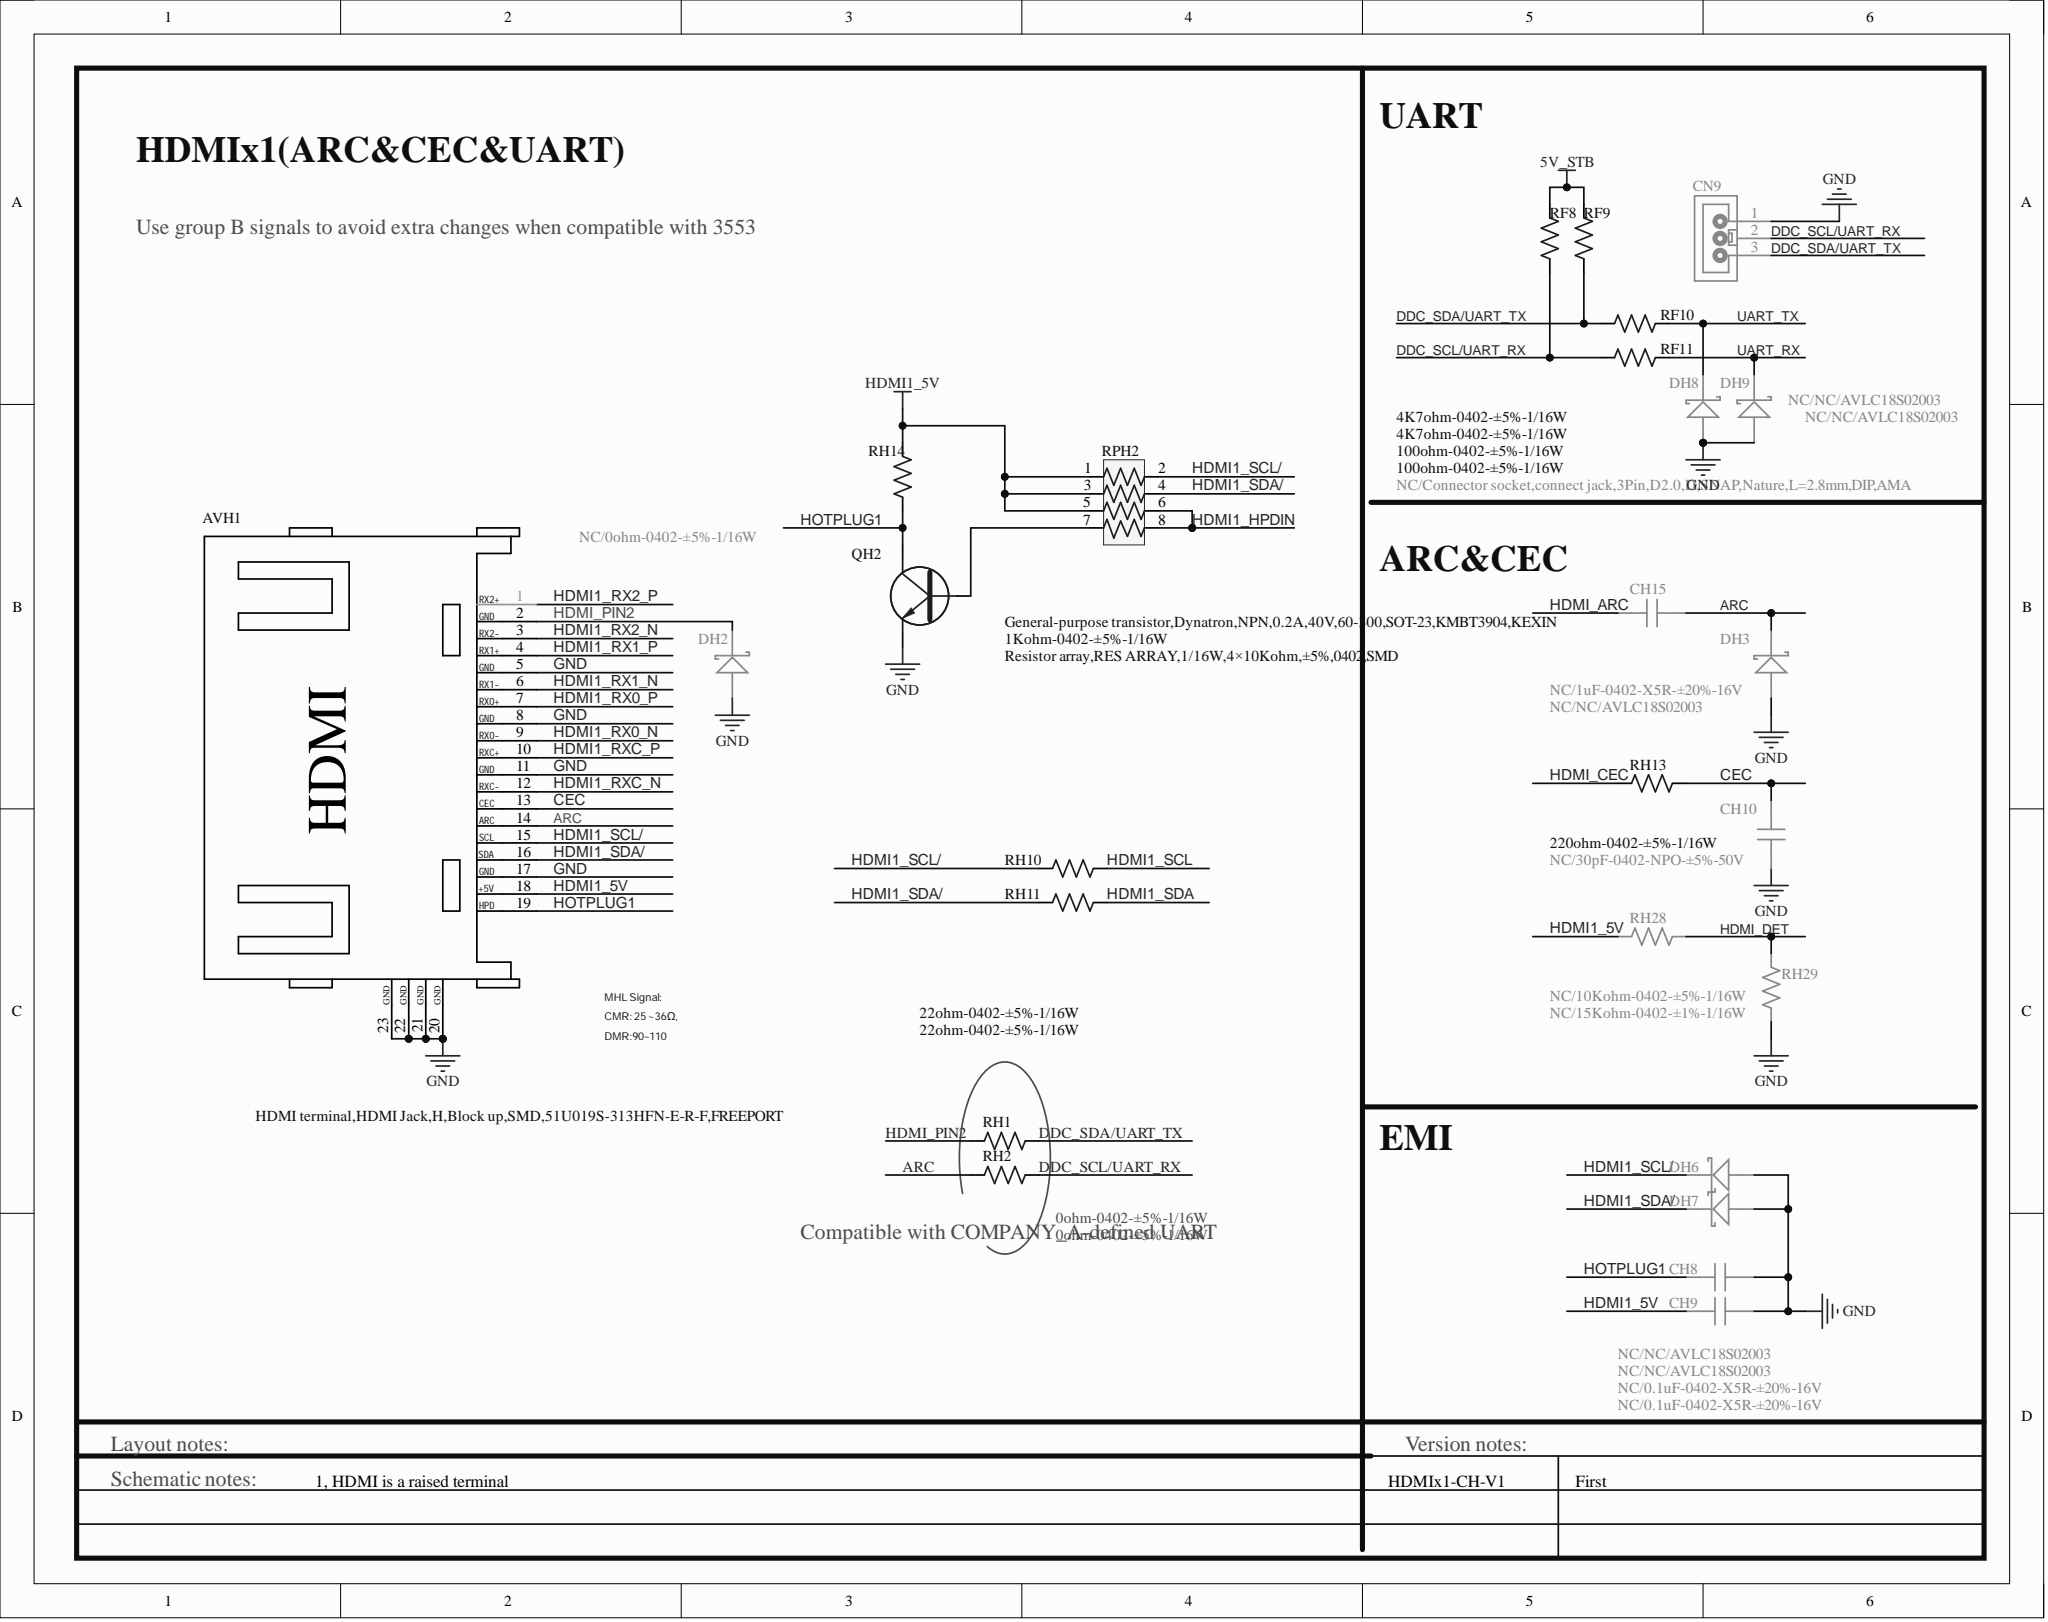Circuit board | Altium Designer | 574 parts | 274 nets | one sheet of the schematic
Parts on this sheet (reference | value | footprint):
AVH1 | HDMI terminal,HDMI Jack,H,Block up,SMD,51U019S-313HFN-E-R-F,FREEPORT | HDMI-HS-11
CH8 | NC/0.1uF-0402-X5R-±20%-16V | C0402
CH9 | NC/0.1uF-0402-X5R-±20%-16V | C0402
CH10 | NC/30pF-0402-NPO-±5%-50V | C0402
CH15 | NC/1uF-0402-X5R-±20%-16V | C0402
CN9 | NC/Connector socket,connect jack,3Pin,D2.0,D,SNAP,Nature,L=2.8mm,DIP,AMA | SIP3/2.0D-3
DH2 | NC/0ohm-0402-±5%-1/16W | DIODE-S0402
DH3 | NC/NC/AVLC18S02003 | DIODE-S0402
DH6 | NC/NC/AVLC18S02003 | DIODE-S0402
DH7 | NC/NC/AVLC18S02003 | DIODE-S0402
DH8 | NC/NC/AVLC18S02003 | DIODE-S0402
DH9 | NC/NC/AVLC18S02003 | DIODE-S0402
QH2 | General-purpose transistor,Dynatron,NPN,0.2A,40V,60-300,SOT-23,KMBT3904,KEXIN | SOT-23
RF8 | 4K7ohm-0402-±5%-1/16W | R0402
RF9 | 4K7ohm-0402-±5%-1/16W | R0402
RF10 | 100ohm-0402-±5%-1/16W | R0402
RF11 | 100ohm-0402-±5%-1/16W | R0402
RH1 | 0ohm-0402-±5%-1/16W | R0402
RH2 | 0ohm-0402-±5%-1/16W | R0402
RH10 | 22ohm-0402-±5%-1/16W | R0402
RH11 | 22ohm-0402-±5%-1/16W | R0402
RH14 | 1Kohm-0402-±5%-1/16W | R0402
RH28 | NC/10Kohm-0402-±5%-1/16W | R0402
RH29 | NC/15Kohm-0402-±1%-1/16W | R0402
RPH2 | Resistor array,RES ARRAY,1/16W,4×10Kohm,±5%,0402,SMD | RA0402
Nets of these parts (net: part-pin ...):
UART_TX: DH8-K RF10-2
UART_RX: DH9-K RF11-2
NetQH2_B: QH2-B RPH2-7
HOTPLUG1: CH8-2 QH2-C RH14-1 AVH1-19
HDMI_PIN2: DH2-K RH1-1 AVH1-2
HDMI_DET: RH28-1 RH29-1
HDMI_ARC: CH15-2
HDMI1_SDA/: DH7-K RH11-2 RPH2-4 AVH1-16
HDMI1_SDA: RH11-1
HDMI1_SCL/: DH6-K RH10-2 RPH2-2 AVH1-15
HDMI1_SCL: RH10-1
HDMI1_RXC_P: AVH1-10
HDMI1_RXC_N: AVH1-12
HDMI1_RX2_P: AVH1-1
HDMI1_RX2_N: AVH1-3
HDMI1_RX1_P: AVH1-4
HDMI1_RX1_N: AVH1-6
HDMI1_RX0_P: AVH1-7
HDMI1_RX0_N: AVH1-9
HDMI1_HPDIN: RPH2-6 RPH2-8
HDMI1_5V: CH9-2 RH14-2 RH28-2 RPH2-1 RPH2-3 RPH2-5 AVH1-18
GND: CH8-1 CH9-1 CH10-1 CN9-1 DH2-A DH3-A DH6-A DH7-A DH8-A DH9-A QH2-E RH29-2 AVH1-5 AVH1-8 AVH1-11 AVH1-17 AVH1-20 AVH1-21 AVH1-22 AVH1-23
DDC_SDA/UART_TX: CN9-3 RF9-1 RF10-1 RH1-2
DDC_SCL/UART_RX: CN9-2 RF8-1 RF11-1 RH2-2
CEC: CH10-2 AVH1-13
ARC: CH15-1 DH3-K RH2-1 AVH1-14
5V_STB: RF8-2 RF9-2